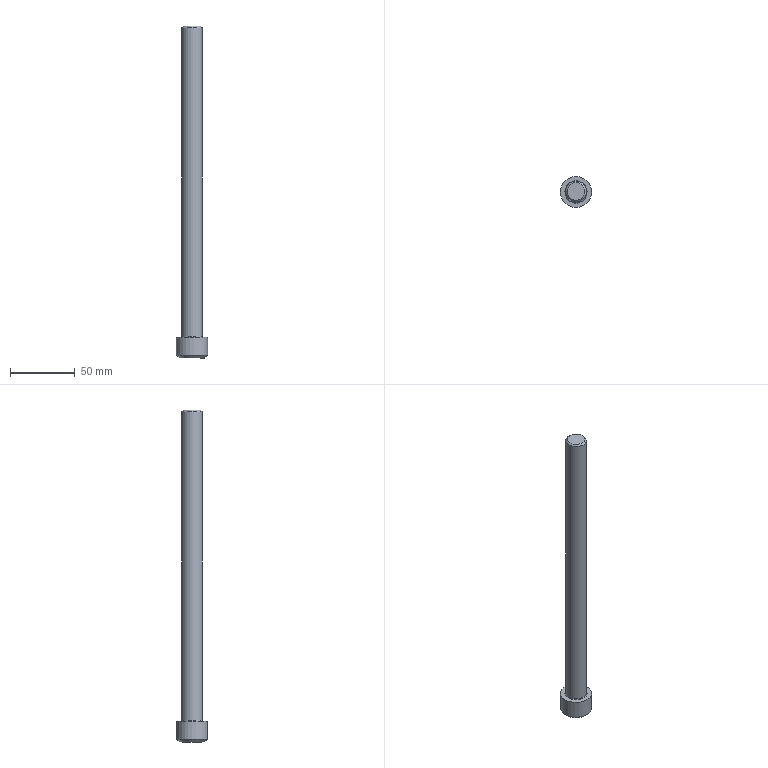Part | NX | features MAIN_BODY 2 | 1 solid | 20 faces | box 24 x 24 x 256 mm | volume 53557 mm3 | plane 11 | cone 5 | cylinder 3 | torus 1 | commonest cylinder face diameters 14 x1 16 x1 24 x1
STEP:
#1=CARTESIAN_POINT('',(-193.,-358.5,148.));
#2=VERTEX_POINT('',#1);
#3=CARTESIAN_POINT('',(-205.,-358.5,148.));
#4=DIRECTION('',(0.,0.,1.));
#5=DIRECTION('',(1.,0.,0.));
#6=AXIS2_PLACEMENT_3D('',#3,#4,#5);
#7=CIRCLE('',#6,12.);
#8=EDGE_CURVE('',#2,#2,#7,.F.);
#9=ORIENTED_EDGE('',*,*,#8,.F.);
#10=EDGE_LOOP('',(#9));
#11=FACE_BOUND('',#10,.T.);
#12=CARTESIAN_POINT('',(-217.,-358.5,162.));
#13=VERTEX_POINT('',#12);
#14=CARTESIAN_POINT('',(-205.,-358.5,162.));
#15=DIRECTION('',(0.,0.,-1.));
#16=DIRECTION('',(-1.,0.,0.));
#17=AXIS2_PLACEMENT_3D('',#14,#15,#16);
#18=CIRCLE('',#17,12.);
#19=EDGE_CURVE('',#13,#13,#18,.T.);
#20=ORIENTED_EDGE('',*,*,#19,.T.);
#21=EDGE_LOOP('',(#20));
#22=FACE_BOUND('',#21,.T.);
#23=CARTESIAN_POINT('',(-205.,-358.5,154.));
#24=DIRECTION('',(0.,0.,-1.));
#25=DIRECTION('',(1.,0.,0.));
#26=AXIS2_PLACEMENT_3D('',#23,#24,#25);
#27=CYLINDRICAL_SURFACE('',#26,12.);
#28=ADVANCED_FACE('',(#11,#22),#27,.T.);
#29=CARTESIAN_POINT('',(-205.,-350.4,146.));
#30=VERTEX_POINT('',#29);
#31=CARTESIAN_POINT('',(-205.,-366.6,146.));
#32=VERTEX_POINT('',#31);
#33=CARTESIAN_POINT('',(-205.,-358.5,146.));
#34=DIRECTION('',(0.,0.,1.));
#35=DIRECTION('',(1.,0.,0.));
#36=AXIS2_PLACEMENT_3D('',#33,#34,#35);
#37=CIRCLE('',#36,8.1);
#38=EDGE_CURVE('',#30,#32,#37,.T.);
#39=ORIENTED_EDGE('',*,*,#38,.T.);
#40=CARTESIAN_POINT('',(-205.,-358.5,146.));
#41=DIRECTION('',(0.,0.,-1.));
#42=DIRECTION('',(-1.,0.,0.));
#43=AXIS2_PLACEMENT_3D('',#40,#41,#42);
#44=CIRCLE('',#43,8.1);
#45=EDGE_CURVE('',#30,#32,#44,.T.);
#46=ORIENTED_EDGE('',*,*,#45,.F.);
#47=EDGE_LOOP('',(#39,#46));
#48=FACE_BOUND('',#47,.T.);
#49=CARTESIAN_POINT('',(-195.,-358.5,146.));
#50=VERTEX_POINT('',#49);
#51=CARTESIAN_POINT('',(-205.,-358.5,146.));
#52=DIRECTION('',(0.,0.,1.));
#53=DIRECTION('',(1.,0.,0.));
#54=AXIS2_PLACEMENT_3D('',#51,#52,#53);
#55=CIRCLE('',#54,10.);
#56=EDGE_CURVE('',#50,#50,#55,.T.);
#57=ORIENTED_EDGE('',*,*,#56,.F.);
#58=EDGE_LOOP('',(#57));
#59=FACE_BOUND('',#58,.T.);
#60=CARTESIAN_POINT('',(-205.,-358.5,146.));
#61=DIRECTION('',(0.,0.,-1.));
#62=DIRECTION('',(1.,0.,0.));
#63=AXIS2_PLACEMENT_3D('',#60,#61,#62);
#64=PLANE('',#63);
#65=ADVANCED_FACE('',(#48,#59),#64,.T.);
#66=CARTESIAN_POINT('',(-213.6,-358.5,162.));
#67=VERTEX_POINT('',#66);
#68=CARTESIAN_POINT('',(-205.,-358.5,162.));
#69=DIRECTION('',(0.,0.,-1.));
#70=DIRECTION('',(-1.,0.,0.));
#71=AXIS2_PLACEMENT_3D('',#68,#69,#70);
#72=CIRCLE('',#71,8.6);
#73=EDGE_CURVE('',#67,#67,#72,.F.);
#74=ORIENTED_EDGE('',*,*,#73,.F.);
#75=EDGE_LOOP('',(#74));
#76=FACE_BOUND('',#75,.T.);
#77=ORIENTED_EDGE('',*,*,#19,.F.);
#78=EDGE_LOOP('',(#77));
#79=FACE_BOUND('',#78,.T.);
#80=CARTESIAN_POINT('',(-205.,-358.5,162.));
#81=DIRECTION('',(0.,0.,1.));
#82=DIRECTION('',(-1.,0.,0.));
#83=AXIS2_PLACEMENT_3D('',#80,#81,#82);
#84=PLANE('',#83);
#85=ADVANCED_FACE('',(#76,#79),#84,.T.);
#86=CARTESIAN_POINT('',(-211.8,-358.5,402.));
#87=VERTEX_POINT('',#86);
#88=CARTESIAN_POINT('',(-205.,-358.5,402.));
#89=DIRECTION('',(0.,0.,-1.));
#90=DIRECTION('',(-1.,0.,0.));
#91=AXIS2_PLACEMENT_3D('',#88,#89,#90);
#92=CIRCLE('',#91,6.8);
#93=EDGE_CURVE('',#87,#87,#92,.T.);
#94=ORIENTED_EDGE('',*,*,#93,.F.);
#95=EDGE_LOOP('',(#94));
#96=FACE_BOUND('',#95,.T.);
#97=CARTESIAN_POINT('',(-205.,-358.5,402.));
#98=DIRECTION('',(0.,0.,1.));
#99=DIRECTION('',(-1.,0.,0.));
#100=AXIS2_PLACEMENT_3D('',#97,#98,#99);
#101=PLANE('',#100);
#102=ADVANCED_FACE('',(#96),#101,.T.);
#103=CARTESIAN_POINT('',(-213.,-358.5,162.6));
#104=VERTEX_POINT('',#103);
#105=CARTESIAN_POINT('',(-205.,-358.5,162.6));
#106=DIRECTION('',(0.,0.,-1.));
#107=DIRECTION('',(-1.,0.,0.));
#108=AXIS2_PLACEMENT_3D('',#105,#106,#107);
#109=CIRCLE('',#108,8.);
#110=EDGE_CURVE('',#104,#104,#109,.T.);
#111=ORIENTED_EDGE('',*,*,#110,.F.);
#112=EDGE_LOOP('',(#111));
#113=FACE_BOUND('',#112,.T.);
#114=CARTESIAN_POINT('',(-213.,-358.5,400.8));
#115=VERTEX_POINT('',#114);
#116=CARTESIAN_POINT('',(-205.,-358.5,400.8));
#117=DIRECTION('',(0.,0.,-1.));
#118=DIRECTION('',(-1.,0.,0.));
#119=AXIS2_PLACEMENT_3D('',#116,#117,#118);
#120=CIRCLE('',#119,8.);
#121=EDGE_CURVE('',#115,#115,#120,.F.);
#122=ORIENTED_EDGE('',*,*,#121,.F.);
#123=EDGE_LOOP('',(#122));
#124=FACE_BOUND('',#123,.T.);
#125=CARTESIAN_POINT('',(-205.,-358.5,162.));
#126=DIRECTION('',(0.,0.,1.));
#127=DIRECTION('',(-1.,0.,0.));
#128=AXIS2_PLACEMENT_3D('',#125,#126,#127);
#129=CYLINDRICAL_SURFACE('',#128,8.);
#130=ADVANCED_FACE('',(#113,#124),#129,.T.);
#131=ORIENTED_EDGE('',*,*,#121,.T.);
#132=EDGE_LOOP('',(#131));
#133=FACE_BOUND('',#132,.T.);
#134=ORIENTED_EDGE('',*,*,#93,.T.);
#135=EDGE_LOOP('',(#134));
#136=FACE_BOUND('',#135,.T.);
#137=CARTESIAN_POINT('',(-205.,-358.5,402.));
#138=DIRECTION('',(0.,0.,-1.));
#139=DIRECTION('',(1.,0.,0.));
#140=AXIS2_PLACEMENT_3D('',#137,#138,#139);
#141=CONICAL_SURFACE('',#140,6.8,0.7854);
#142=ADVANCED_FACE('',(#133,#136),#141,.T.);
#143=ORIENTED_EDGE('',*,*,#8,.T.);
#144=EDGE_LOOP('',(#143));
#145=FACE_BOUND('',#144,.T.);
#146=ORIENTED_EDGE('',*,*,#56,.T.);
#147=EDGE_LOOP('',(#146));
#148=FACE_BOUND('',#147,.T.);
#149=CARTESIAN_POINT('',(-205.,-358.5,146.));
#150=DIRECTION('',(0.,0.,1.));
#151=DIRECTION('',(-1.,0.,0.));
#152=AXIS2_PLACEMENT_3D('',#149,#150,#151);
#153=CONICAL_SURFACE('',#152,10.,0.7854);
#154=ADVANCED_FACE('',(#145,#148),#153,.T.);
#155=ORIENTED_EDGE('',*,*,#73,.T.);
#156=EDGE_LOOP('',(#155));
#157=FACE_BOUND('',#156,.T.);
#158=ORIENTED_EDGE('',*,*,#110,.T.);
#159=EDGE_LOOP('',(#158));
#160=FACE_BOUND('',#159,.T.);
#161=CARTESIAN_POINT('',(-205.,-358.5,162.6));
#162=DIRECTION('',(0.,0.,1.));
#163=DIRECTION('',(-1.,0.,0.));
#164=AXIS2_PLACEMENT_3D('',#161,#162,#163);
#165=TOROIDAL_SURFACE('',#164,8.6,0.6);
#166=ADVANCED_FACE('',(#157,#160),#165,.F.);
#167=CARTESIAN_POINT('',(-198.,-362.559,146.005));
#168=VERTEX_POINT('',#167);
#169=CARTESIAN_POINT('',(-205.,-366.6,146.));
#170=CARTESIAN_POINT('',(-203.857,-365.94,146.381));
#171=CARTESIAN_POINT('',(-201.513,-364.587,146.87));
#172=CARTESIAN_POINT('',(-199.145,-363.219,146.385));
#173=CARTESIAN_POINT('',(-198.,-362.559,146.005));
#174=B_SPLINE_CURVE_WITH_KNOTS('',3,(#169,#170,#171,#172,#173),.UNSPECIFIED.,.F.,.F.,(4,1,4),(0.000000238,0.004082,0.008163),.UNSPECIFIED.);
#175=EDGE_CURVE('',#32,#168,#174,.T.);
#176=ORIENTED_EDGE('',*,*,#175,.T.);
#177=CARTESIAN_POINT('',(-198.,-354.441,146.005));
#178=VERTEX_POINT('',#177);
#179=CARTESIAN_POINT('',(-198.,-362.559,146.005));
#180=CARTESIAN_POINT('',(-198.,-361.24,146.387));
#181=CARTESIAN_POINT('',(-198.,-358.501,146.884));
#182=CARTESIAN_POINT('',(-198.,-355.753,146.385));
#183=CARTESIAN_POINT('',(-198.,-354.441,146.005));
#184=B_SPLINE_CURVE_WITH_KNOTS('',3,(#179,#180,#181,#182,#183),.UNSPECIFIED.,.F.,.F.,(4,1,4),(0.00695,0.01105,0.01516),.UNSPECIFIED.);
#185=EDGE_CURVE('',#168,#178,#184,.T.);
#186=ORIENTED_EDGE('',*,*,#185,.T.);
#187=CARTESIAN_POINT('',(-198.,-354.441,146.005));
#188=CARTESIAN_POINT('',(-199.143,-353.781,146.385));
#189=CARTESIAN_POINT('',(-201.488,-352.428,146.87));
#190=CARTESIAN_POINT('',(-203.856,-351.061,146.381));
#191=CARTESIAN_POINT('',(-205.,-350.4,146.));
#192=B_SPLINE_CURVE_WITH_KNOTS('',3,(#187,#188,#189,#190,#191),.UNSPECIFIED.,.F.,.F.,(4,1,4),(0.000000238,0.004082,0.008163),.UNSPECIFIED.);
#193=EDGE_CURVE('',#178,#30,#192,.T.);
#194=ORIENTED_EDGE('',*,*,#193,.T.);
#195=ORIENTED_EDGE('',*,*,#45,.T.);
#196=EDGE_LOOP('',(#176,#186,#194,#195));
#197=FACE_BOUND('',#196,.T.);
#198=CARTESIAN_POINT('',(-205.,-358.5,150.677));
#199=DIRECTION('',(0.,0.,-1.));
#200=DIRECTION('',(1.,0.,0.));
#201=AXIS2_PLACEMENT_3D('',#198,#199,#200);
#202=CONICAL_SURFACE('',#201,0.,1.047);
#203=ADVANCED_FACE('',(#197),#202,.F.);
#204=CARTESIAN_POINT('',(-212.,-354.441,146.005));
#205=VERTEX_POINT('',#204);
#206=CARTESIAN_POINT('',(-212.,-362.559,146.005));
#207=VERTEX_POINT('',#206);
#208=CARTESIAN_POINT('',(-212.,-362.559,146.005));
#209=CARTESIAN_POINT('',(-212.,-361.24,146.387));
#210=CARTESIAN_POINT('',(-212.,-358.501,146.884));
#211=CARTESIAN_POINT('',(-212.,-355.753,146.385));
#212=CARTESIAN_POINT('',(-212.,-354.441,146.005));
#213=B_SPLINE_CURVE_WITH_KNOTS('',3,(#208,#209,#210,#211,#212),.UNSPECIFIED.,.F.,.F.,(4,1,4),(0.00695,0.01105,0.01516),.UNSPECIFIED.);
#214=EDGE_CURVE('',#205,#207,#213,.F.);
#215=ORIENTED_EDGE('',*,*,#214,.T.);
#216=CARTESIAN_POINT('',(-212.,-362.559,146.005));
#217=CARTESIAN_POINT('',(-210.857,-363.219,146.385));
#218=CARTESIAN_POINT('',(-208.512,-364.572,146.87));
#219=CARTESIAN_POINT('',(-206.144,-365.939,146.381));
#220=CARTESIAN_POINT('',(-205.,-366.6,146.));
#221=B_SPLINE_CURVE_WITH_KNOTS('',3,(#216,#217,#218,#219,#220),.UNSPECIFIED.,.F.,.F.,(4,1,4),(0.000000238,0.004082,0.008163),.UNSPECIFIED.);
#222=EDGE_CURVE('',#207,#32,#221,.T.);
#223=ORIENTED_EDGE('',*,*,#222,.T.);
#224=ORIENTED_EDGE('',*,*,#38,.F.);
#225=CARTESIAN_POINT('',(-212.,-354.441,146.005));
#226=CARTESIAN_POINT('',(-210.857,-353.781,146.385));
#227=CARTESIAN_POINT('',(-208.512,-352.428,146.87));
#228=CARTESIAN_POINT('',(-206.144,-351.061,146.381));
#229=CARTESIAN_POINT('',(-205.,-350.4,146.));
#230=B_SPLINE_CURVE_WITH_KNOTS('',3,(#225,#226,#227,#228,#229),.UNSPECIFIED.,.F.,.F.,(4,1,4),(0.000000238,0.004082,0.008163),.UNSPECIFIED.);
#231=EDGE_CURVE('',#205,#30,#230,.T.);
#232=ORIENTED_EDGE('',*,*,#231,.F.);
#233=EDGE_LOOP('',(#215,#223,#224,#232));
#234=FACE_BOUND('',#233,.T.);
#235=CARTESIAN_POINT('',(-205.,-358.5,150.677));
#236=DIRECTION('',(0.,0.,-1.));
#237=DIRECTION('',(1.,0.,0.));
#238=AXIS2_PLACEMENT_3D('',#235,#236,#237);
#239=CONICAL_SURFACE('',#238,0.,1.047);
#240=ADVANCED_FACE('',(#234),#239,.F.);
#241=CARTESIAN_POINT('',(-212.,-358.5,155.2));
#242=VERTEX_POINT('',#241);
#243=CARTESIAN_POINT('',(-205.,-358.5,155.2));
#244=DIRECTION('',(0.,0.,-1.));
#245=DIRECTION('',(-1.,0.,0.));
#246=AXIS2_PLACEMENT_3D('',#243,#244,#245);
#247=CIRCLE('',#246,7.);
#248=EDGE_CURVE('',#242,#242,#247,.T.);
#249=ORIENTED_EDGE('',*,*,#248,.T.);
#250=EDGE_LOOP('',(#249));
#251=FACE_BOUND('',#250,.T.);
#252=CARTESIAN_POINT('',(-205.,-358.5,159.241));
#253=VERTEX_POINT('',#252);
#254=VERTEX_LOOP('',#253);
#255=FACE_BOUND('',#254,.T.);
#256=CARTESIAN_POINT('',(-205.,-358.5,155.2));
#257=DIRECTION('',(0.,0.,-1.));
#258=DIRECTION('',(1.,0.,0.));
#259=AXIS2_PLACEMENT_3D('',#256,#257,#258);
#260=CONICAL_SURFACE('',#259,7.,1.047);
#261=ADVANCED_FACE('',(#251,#255),#260,.F.);
#262=ORIENTED_EDGE('',*,*,#248,.F.);
#263=EDGE_LOOP('',(#262));
#264=FACE_BOUND('',#263,.T.);
#265=CARTESIAN_POINT('',(-212.,-358.5,154.));
#266=VERTEX_POINT('',#265);
#267=CARTESIAN_POINT('',(-198.,-358.5,154.));
#268=VERTEX_POINT('',#267);
#269=CARTESIAN_POINT('',(-205.,-358.5,154.));
#270=DIRECTION('',(0.,0.,-1.));
#271=DIRECTION('',(-1.,0.,0.));
#272=AXIS2_PLACEMENT_3D('',#269,#270,#271);
#273=CIRCLE('',#272,7.);
#274=EDGE_CURVE('',#266,#268,#273,.T.);
#275=ORIENTED_EDGE('',*,*,#274,.T.);
#276=CARTESIAN_POINT('',(-205.,-358.5,154.));
#277=DIRECTION('',(0.,0.,-1.));
#278=DIRECTION('',(-1.,0.,0.));
#279=AXIS2_PLACEMENT_3D('',#276,#277,#278);
#280=CIRCLE('',#279,7.);
#281=EDGE_CURVE('',#268,#266,#280,.T.);
#282=ORIENTED_EDGE('',*,*,#281,.T.);
#283=EDGE_LOOP('',(#275,#282));
#284=FACE_BOUND('',#283,.T.);
#285=CARTESIAN_POINT('',(-205.,-358.5,154.));
#286=DIRECTION('',(0.,0.,1.));
#287=DIRECTION('',(-1.,0.,0.));
#288=AXIS2_PLACEMENT_3D('',#285,#286,#287);
#289=CYLINDRICAL_SURFACE('',#288,7.);
#290=ADVANCED_FACE('',(#264,#284),#289,.F.);
#291=CARTESIAN_POINT('',(-198.,-362.559,154.));
#292=VERTEX_POINT('',#291);
#293=CARTESIAN_POINT('',(-198.,-362.559,154.));
#294=DIRECTION('',(0.,1.,0.));
#295=VECTOR('',#294,1000.);
#296=LINE('',#293,#295);
#297=EDGE_CURVE('',#292,#268,#296,.T.);
#298=ORIENTED_EDGE('',*,*,#297,.F.);
#299=CARTESIAN_POINT('',(-205.,-366.6,154.));
#300=VERTEX_POINT('',#299);
#301=CARTESIAN_POINT('',(-205.,-366.6,154.));
#302=DIRECTION('',(0.866,0.5,0.));
#303=VECTOR('',#302,1000.);
#304=LINE('',#301,#303);
#305=EDGE_CURVE('',#300,#292,#304,.T.);
#306=ORIENTED_EDGE('',*,*,#305,.F.);
#307=CARTESIAN_POINT('',(-212.,-362.559,154.));
#308=VERTEX_POINT('',#307);
#309=CARTESIAN_POINT('',(-212.,-362.559,154.));
#310=DIRECTION('',(0.866,-0.5,0.));
#311=VECTOR('',#310,1000.);
#312=LINE('',#309,#311);
#313=EDGE_CURVE('',#308,#300,#312,.T.);
#314=ORIENTED_EDGE('',*,*,#313,.F.);
#315=CARTESIAN_POINT('',(-212.,-354.441,154.));
#316=DIRECTION('',(0.,-1.,0.));
#317=VECTOR('',#316,1000.);
#318=LINE('',#315,#317);
#319=EDGE_CURVE('',#266,#308,#318,.T.);
#320=ORIENTED_EDGE('',*,*,#319,.F.);
#321=ORIENTED_EDGE('',*,*,#281,.F.);
#322=EDGE_LOOP('',(#298,#306,#314,#320,#321));
#323=FACE_BOUND('',#322,.T.);
#324=CARTESIAN_POINT('',(-205.,-358.5,154.));
#325=DIRECTION('',(0.,0.,-1.));
#326=DIRECTION('',(1.,0.,0.));
#327=AXIS2_PLACEMENT_3D('',#324,#325,#326);
#328=PLANE('',#327);
#329=ADVANCED_FACE('',(#323),#328,.T.);
#330=CARTESIAN_POINT('',(-212.,-354.441,154.));
#331=VERTEX_POINT('',#330);
#332=CARTESIAN_POINT('',(-212.,-354.441,154.));
#333=DIRECTION('',(0.,-1.,0.));
#334=VECTOR('',#333,1000.);
#335=LINE('',#332,#334);
#336=EDGE_CURVE('',#331,#266,#335,.T.);
#337=ORIENTED_EDGE('',*,*,#336,.F.);
#338=CARTESIAN_POINT('',(-205.,-350.4,154.));
#339=VERTEX_POINT('',#338);
#340=CARTESIAN_POINT('',(-212.,-354.441,154.));
#341=DIRECTION('',(0.866,0.5,0.));
#342=VECTOR('',#341,1000.);
#343=LINE('',#340,#342);
#344=EDGE_CURVE('',#331,#339,#343,.T.);
#345=ORIENTED_EDGE('',*,*,#344,.T.);
#346=CARTESIAN_POINT('',(-198.,-354.441,154.));
#347=VERTEX_POINT('',#346);
#348=CARTESIAN_POINT('',(-198.,-354.441,154.));
#349=DIRECTION('',(-0.866,0.5,0.));
#350=VECTOR('',#349,1000.);
#351=LINE('',#348,#350);
#352=EDGE_CURVE('',#347,#339,#351,.T.);
#353=ORIENTED_EDGE('',*,*,#352,.F.);
#354=CARTESIAN_POINT('',(-198.,-362.559,154.));
#355=DIRECTION('',(0.,1.,0.));
#356=VECTOR('',#355,1000.);
#357=LINE('',#354,#356);
#358=EDGE_CURVE('',#268,#347,#357,.T.);
#359=ORIENTED_EDGE('',*,*,#358,.F.);
#360=ORIENTED_EDGE('',*,*,#274,.F.);
#361=EDGE_LOOP('',(#337,#345,#353,#359,#360));
#362=FACE_BOUND('',#361,.T.);
#363=CARTESIAN_POINT('',(-205.,-358.5,154.));
#364=DIRECTION('',(0.,0.,-1.));
#365=DIRECTION('',(1.,0.,0.));
#366=AXIS2_PLACEMENT_3D('',#363,#364,#365);
#367=PLANE('',#366);
#368=ADVANCED_FACE('',(#362),#367,.T.);
#369=CARTESIAN_POINT('',(-198.,-354.441,154.));
#370=DIRECTION('',(0.,0.,-1.));
#371=VECTOR('',#370,1000.);
#372=LINE('',#369,#371);
#373=EDGE_CURVE('',#347,#178,#372,.T.);
#374=ORIENTED_EDGE('',*,*,#373,.F.);
#375=ORIENTED_EDGE('',*,*,#352,.T.);
#376=CARTESIAN_POINT('',(-205.,-350.4,154.));
#377=DIRECTION('',(0.,0.,-1.));
#378=VECTOR('',#377,1000.);
#379=LINE('',#376,#378);
#380=EDGE_CURVE('',#339,#30,#379,.T.);
#381=ORIENTED_EDGE('',*,*,#380,.T.);
#382=ORIENTED_EDGE('',*,*,#193,.F.);
#383=EDGE_LOOP('',(#374,#375,#381,#382));
#384=FACE_BOUND('',#383,.T.);
#385=CARTESIAN_POINT('',(-198.,-354.441,154.));
#386=DIRECTION('',(0.5,0.866,0.));
#387=DIRECTION('',(-0.866,0.5,0.));
#388=AXIS2_PLACEMENT_3D('',#385,#386,#387);
#389=PLANE('',#388);
#390=ADVANCED_FACE('',(#384),#389,.F.);
#391=ORIENTED_EDGE('',*,*,#231,.T.);
#392=ORIENTED_EDGE('',*,*,#380,.F.);
#393=ORIENTED_EDGE('',*,*,#344,.F.);
#394=CARTESIAN_POINT('',(-212.,-354.441,154.));
#395=DIRECTION('',(0.,0.,-1.));
#396=VECTOR('',#395,1000.);
#397=LINE('',#394,#396);
#398=EDGE_CURVE('',#331,#205,#397,.T.);
#399=ORIENTED_EDGE('',*,*,#398,.T.);
#400=EDGE_LOOP('',(#391,#392,#393,#399));
#401=FACE_BOUND('',#400,.T.);
#402=CARTESIAN_POINT('',(-212.,-354.441,154.));
#403=DIRECTION('',(0.5,-0.866,0.));
#404=DIRECTION('',(0.866,0.5,0.));
#405=AXIS2_PLACEMENT_3D('',#402,#403,#404);
#406=PLANE('',#405);
#407=ADVANCED_FACE('',(#401),#406,.T.);
#408=ORIENTED_EDGE('',*,*,#398,.F.);
#409=ORIENTED_EDGE('',*,*,#336,.T.);
#410=ORIENTED_EDGE('',*,*,#319,.T.);
#411=CARTESIAN_POINT('',(-212.,-362.559,154.));
#412=DIRECTION('',(0.,0.,-1.));
#413=VECTOR('',#412,1000.);
#414=LINE('',#411,#413);
#415=EDGE_CURVE('',#308,#207,#414,.T.);
#416=ORIENTED_EDGE('',*,*,#415,.T.);
#417=ORIENTED_EDGE('',*,*,#214,.F.);
#418=EDGE_LOOP('',(#408,#409,#410,#416,#417));
#419=FACE_BOUND('',#418,.T.);
#420=CARTESIAN_POINT('',(-212.,-354.441,154.));
#421=DIRECTION('',(-1.,0.,0.));
#422=DIRECTION('',(0.,-1.,0.));
#423=AXIS2_PLACEMENT_3D('',#420,#421,#422);
#424=PLANE('',#423);
#425=ADVANCED_FACE('',(#419),#424,.F.);
#426=ORIENTED_EDGE('',*,*,#415,.F.);
#427=ORIENTED_EDGE('',*,*,#313,.T.);
#428=CARTESIAN_POINT('',(-205.,-366.6,154.));
#429=DIRECTION('',(0.,0.,-1.));
#430=VECTOR('',#429,1000.);
#431=LINE('',#428,#430);
#432=EDGE_CURVE('',#300,#32,#431,.T.);
#433=ORIENTED_EDGE('',*,*,#432,.T.);
#434=ORIENTED_EDGE('',*,*,#222,.F.);
#435=EDGE_LOOP('',(#426,#427,#433,#434));
#436=FACE_BOUND('',#435,.T.);
#437=CARTESIAN_POINT('',(-212.,-362.559,154.));
#438=DIRECTION('',(-0.5,-0.866,0.));
#439=DIRECTION('',(0.866,-0.5,0.));
#440=AXIS2_PLACEMENT_3D('',#437,#438,#439);
#441=PLANE('',#440);
#442=ADVANCED_FACE('',(#436),#441,.F.);
#443=ORIENTED_EDGE('',*,*,#432,.F.);
#444=ORIENTED_EDGE('',*,*,#305,.T.);
#445=CARTESIAN_POINT('',(-198.,-362.559,154.));
#446=DIRECTION('',(0.,0.,-1.));
#447=VECTOR('',#446,1000.);
#448=LINE('',#445,#447);
#449=EDGE_CURVE('',#292,#168,#448,.T.);
#450=ORIENTED_EDGE('',*,*,#449,.T.);
#451=ORIENTED_EDGE('',*,*,#175,.F.);
#452=EDGE_LOOP('',(#443,#444,#450,#451));
#453=FACE_BOUND('',#452,.T.);
#454=CARTESIAN_POINT('',(-205.,-366.6,154.));
#455=DIRECTION('',(0.5,-0.866,0.));
#456=DIRECTION('',(0.866,0.5,0.));
#457=AXIS2_PLACEMENT_3D('',#454,#455,#456);
#458=PLANE('',#457);
#459=ADVANCED_FACE('',(#453),#458,.F.);
#460=ORIENTED_EDGE('',*,*,#449,.F.);
#461=ORIENTED_EDGE('',*,*,#297,.T.);
#462=ORIENTED_EDGE('',*,*,#358,.T.);
#463=ORIENTED_EDGE('',*,*,#373,.T.);
#464=ORIENTED_EDGE('',*,*,#185,.F.);
#465=EDGE_LOOP('',(#460,#461,#462,#463,#464));
#466=FACE_BOUND('',#465,.T.);
#467=CARTESIAN_POINT('',(-198.,-362.559,154.));
#468=DIRECTION('',(1.,0.,0.));
#469=DIRECTION('',(0.,0.,1.));
#470=AXIS2_PLACEMENT_3D('',#467,#468,#469);
#471=PLANE('',#470);
#472=ADVANCED_FACE('',(#466),#471,.F.);
#473=CLOSED_SHELL('',(#28,#65,#85,#102,#130,#142,#154,#166,#203,#240,#261,#290,#329,#368,#390,#407,#425,#442,#459,#472));
#474=MANIFOLD_SOLID_BREP('',#473);
#475=(LENGTH_UNIT()NAMED_UNIT(*)SI_UNIT(.MILLI.,.METRE.));
#476=UNCERTAINTY_MEASURE_WITH_UNIT(LENGTH_MEASURE(0.0508),#475,'','');
#477=(NAMED_UNIT(*)PLANE_ANGLE_UNIT()SI_UNIT($,.RADIAN.));
#478=(NAMED_UNIT(*)SI_UNIT($,.STERADIAN.)SOLID_ANGLE_UNIT());
#479=(GEOMETRIC_REPRESENTATION_CONTEXT(3)GLOBAL_UNCERTAINTY_ASSIGNED_CONTEXT((#476))GLOBAL_UNIT_ASSIGNED_CONTEXT((#475,#477,#478))REPRESENTATION_CONTEXT('',''));
#480=ADVANCED_BREP_SHAPE_REPRESENTATION('',(#474),#479);